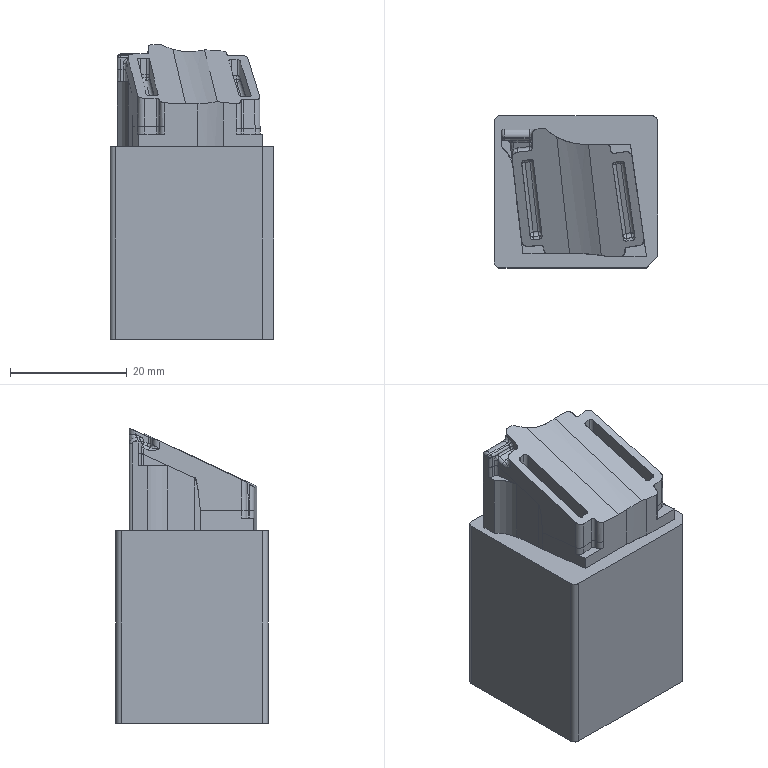NC program | NX | posted with a generic post | part box 28 x 26 x 50.455 mm
Lines 1 to 1095 of 4248:
N10 G17 G21 G94 G90
(CAVITY_MILL , TOOL : D6)
N12 T00 M6
N14 G54
N16 G17 G0 G90 X5.189 Y-18.995 S0 M3
N18 G43 Z10. H0
N20 Z-0.048
N22 G94 G1 Z-0.348 F250.
N24 Y-16.295
N26 G3 X2.189 Y-13.295 R3.
N28 G1 X-14.003
N30 G2 X-14.296 Y-13.002 R0.293
N32 G1 Y13.007
N34 G2 X-14.008 Y13.295 R0.288
N36 G1 X-10.132
N38 G2 X-6.501 Y14.818 R5.101
N40 G1 X-5.218
N42 G2 X-2.444 Y13.737 R4.1
N44 G3 X-2.084 Y13.432 R5.9
N46 G2 X-1.909 Y13.295 R4.185
N48 G1 X14.005
N50 G2 X14.295 Y13.005 R0.29
N52 G1 Y-13.008
N54 G2 X14.008 Y-13.295 R0.287
N56 G1 X2.189
N58 Y-10.295
N60 X-11.296
N62 Y8.229
N64 G3 X-7.035 Y5.647 R4.178
N66 G1 X-3.905 Y6.01
N68 X-3.886 Y6.012
N70 X-3.675 Y6.043
N72 X-3.539 Y6.08
N74 X-2.274 Y6.586
N76 X-2.149 Y6.654
N78 G3 X-0.393 Y10.295 R4.185
N80 G1 X-0.992 Y10.262
N82 G2 X-2.497 Y7.143 R3.585
N84 G1 X-3.762 Y6.637
N86 X-3.974 Y6.606
N88 X-7.104 Y6.243
N90 G2 X-10.881 Y10.738 R3.578
N92 G1 X-10.873 Y10.762
N94 X-10.85 Y10.862
N96 G2 X-6.501 Y14.218 R4.501
N98 G1 X-5.218
N100 G2 X-2.85 Y13.295 R3.5
N102 G3 X-2.447 Y12.954 R6.5
N104 G2 X-0.992 Y10.262 R3.585
N106 G1 X-0.393 Y10.295
N108 X11.295
N110 Y-10.295
N112 X2.189
N114 Y-7.295
N116 X-8.296
N118 Y2.681
N120 G3 X-6.689 Y2.667 R7.178
N122 G1 X-3.536 Y3.032
N124 X-3.472 Y3.041
N126 X-3.237 Y3.075
N128 G3 X-2.426 Y3.294 R3.6
N130 G1 X-1.16 Y3.8
N132 G3 X-0.412 Y4.208 R3.6
N134 X2.057 Y7.295 R7.185
N136 G1 X8.295
N138 Y-7.295
N140 X2.189
N142 Y-4.295
N144 X-5.296
N146 Y-0.192
N148 X-3.167 Y0.055
N150 X-3.057 Y0.07
N152 X-2.8 Y0.107
N154 G3 X-1.312 Y0.509 R6.6
N156 G1 X-0.046 Y1.015
N158 G3 X1.324 Y1.761 R6.6
N160 X3.82 Y4.295 R10.185
N162 G1 X5.295
N164 Y-4.295
N166 X2.189
N168 Y-1.295
N170 X2.082
N172 G3 X2.295 Y-1.176 R9.6
N174 G1 Y-1.295
N176 X2.189
N178 G3 X-0.811 Y-4.295 R3.
N180 G1 Z-0.048
N182 G0 Z0.3
N184 X3. Y-18.995
N186 Z-0.395
N188 G1 Z-0.695
N190 Y-16.295
N192 G3 X0. Y-13.295 R3.
N194 G1 X-14.003
N196 G2 X-14.296 Y-13.002 R0.293
N198 G1 Y13.007
N200 G2 X-14.008 Y13.295 R0.288
N202 G1 X-10.137
N204 G2 X-6.502 Y14.818 R5.1
N206 G1 X-5.218
N208 G2 X-2.444 Y13.737 R4.1
N210 G3 X-1.902 Y13.295 R5.9
N212 G1 X14.005
N214 G2 X14.295 Y13.005 R0.291
N216 G1 Y-13.008
N218 G2 X14.008 Y-13.295 R0.287
N220 G1 X0.
N222 Y-10.295
N224 X-11.296
N226 Y7.474
N228 G3 X-7.036 Y4.896 R4.166
N230 G1 X-2.8 Y5.387
N232 G3 X0.043 Y7.269 R3.77
N234 X0.495 Y10.295 R4.247
N236 G1 X-0.09 Y10.164
N238 G2 X-0.479 Y7.566 R3.647
N240 X-2.87 Y5.983 R3.17
N242 G1 X-7.105 Y5.492
N244 G2 X-11.002 Y9.102 R3.566
N246 G1 Y9.712
N248 G2 X-6.502 Y14.218 R4.5
N250 G1 X-5.218
N252 G2 X-2.85 Y13.295 R3.5
N254 G3 X-1.843 Y12.536 R6.5
N256 G2 X-0.09 Y10.164 R3.647
N258 G1 X0.495 Y10.295
N260 X11.295
N262 Y-10.295
N264 X0.
N266 Y-7.295
N268 X-8.296
N270 Y1.928
N272 G3 X-6.69 Y1.916 R7.166
N274 G1 X-2.455 Y2.407
N276 G3 X2.651 Y5.786 R6.77
N278 X3.295 Y7.295 R7.247
N280 G1 X8.295
N282 Y-7.295
N284 X0.
N286 Y-4.295
N288 X-5.296
N290 Y-0.942
N292 X-2.109 Y-0.573
N294 G3 X5.254 Y4.295 R9.77
N296 G1 X5.295
N298 Y-4.295
N300 X0.
N302 G3 X-3. Y-7.295 R3.
N304 G1 Y-18.995
N306 Z-0.395
N308 G0 Z-0.048
N310 X3.
N312 Z-0.743
N314 G1 Z-1.043
N316 Y-16.295
N318 G3 X0. Y-13.295 R3.
N320 G1 X-14.003
N322 G2 X-14.296 Y-13.002 R0.293
N324 G1 Y13.007
N326 G2 X-14.008 Y13.295 R0.288
N328 G1 X-10.152
N330 G2 X-6.527 Y14.818 R5.078
N332 G1 X-5.218
N334 G2 X-2.444 Y13.737 R4.1
N336 G3 X-1.902 Y13.295 R5.9
N338 G1 X14.005
N340 G2 X14.295 Y13.005 R0.291
N342 G1 Y-13.008
N344 G2 X14.008 Y-13.295 R0.287
N346 G1 X0.
N348 Y-10.295
N350 X-11.296
N352 Y6.715
N354 G3 X-7.049 Y4.144 R4.158
N356 G1 X-2.772 Y4.64
N358 X-1.197 Y4.728
N360 X-1.175 Y4.73
N362 G3 X2.695 Y3.609 R6.725
N364 G1 X2.767 Y3.615
N366 X5.869 Y4.063
N368 G3 X8.649 Y10.295 R4.048
N370 G1 X8.149 Y9.965
N372 G2 X5.784 Y4.657 R3.448
N374 G1 X2.681 Y4.209
N376 G2 X-1.038 Y5.365 R6.125
N378 G1 X-1.231 Y5.327
N380 X-2.823 Y5.238
N382 X-7.106 Y4.741
N384 G2 X-11.003 Y8.351 R3.558
N386 G1 X-11.004 Y9.735
N388 G2 X-6.527 Y14.218 R4.478
N390 G1 X-5.218
N392 G2 X-2.85 Y13.295 R3.5
N394 G3 X-1.029 Y12.114 R6.5
N396 G2 X0.187 Y11.424 R5.654
N398 G1 X1.3 Y11.576
N400 X1.574 Y11.581
N402 X4.049
N404 G2 X5.73 Y11.483 R10.39
N406 X8.149 Y9.965 R3.448
N408 G1 X8.649 Y10.295
N410 X11.295
N412 Y-10.295
N414 X0.
N416 Y-7.295
N418 X-8.296
N420 Y1.176
N422 G3 X-6.703 Y1.164 R7.158
N424 G1 X-2.515 Y1.65
N426 X-1.903 Y1.684
N428 G3 X2.761 Y0.61 R9.725
N430 X3.196 Y0.646 R3.6
N432 G1 X6.313 Y1.096
N434 G3 X8.295 Y1.701 R7.048
N436 G1 Y-7.295
N438 X0.
N440 Y-4.295
N442 X-5.296
N444 Y-1.693
N446 X-2.466 Y-1.365
N448 G3 X2.828 Y-2.39 R12.725
N450 X3.625 Y-2.324 R6.6
N452 G1 X5.295 Y-2.082
N454 Y-4.295
N456 X0.
N458 G3 X-3. Y-7.295 R3.
N460 G1 Y-18.995
N462 Z-0.743
N464 G0 Z-0.395
N466 X3.
N468 Z-1.091
N470 G1 Z-1.391
N472 Y-16.295
N474 G3 X0. Y-13.295 R3.
N476 G1 X-14.003
N478 G2 X-14.296 Y-13.002 R0.293
N480 G1 Y13.007
N482 G2 X-14.008 Y13.295 R0.288
N484 G1 X-10.241
N486 G2 X-6.557 Y14.818 R5.166
N488 G1 X-5.218
N490 G2 X-2.444 Y13.737 R4.1
N492 G3 X-1.902 Y13.295 R5.9
N494 G1 X14.005
N496 G2 X14.296 Y13.004 R0.291
N498 G1 X14.295 Y-13.008
N500 G2 X14.008 Y-13.295 R0.287
N502 G1 X0.
N504 Y-10.295
N506 X-11.296
N508 Y5.957
N510 G3 X-7.049 Y3.393 R4.154
N512 G1 X-2.681 Y3.9
N514 G2 X0.39 Y3.283 R5.63
N516 G3 X2.853 Y2.871 R4.182
N518 G1 X6.498 Y3.398
N520 G3 X9.902 Y8.337 R4.126
N522 X8.986 Y10.295 R4.882
N524 G1 X8.513 Y9.927
N526 G2 X9.315 Y8.211 R4.282
N528 X6.412 Y3.992 R3.526
N530 G1 X2.767 Y3.465
N532 G2 X0.668 Y3.816 R3.582
N534 G3 X-2.741 Y4.497 R6.23
N536 G1 X-7.118 Y3.989
N538 G2 X-11.004 Y7.6 R3.554
N540 G1 X-11.005 Y8.547
N542 G2 X-10.003 Y12.676 R4.399
N544 G1 X-9.932 Y12.751
N546 G2 X-6.558 Y14.218 R4.566
N548 G1 X-5.218
N550 G2 X-2.85 Y13.295 R3.5
N552 G3 X1.548 Y11.581 R6.5
N554 G1 X5.214
N556 G2 X8.513 Y9.927 R4.282
N558 G1 X8.986 Y10.295
N560 X11.296
N562 X11.295 Y-10.295
N564 X0.
N566 Y-7.295
N568 X-8.296
N570 Y0.424
N572 G3 X-6.73 Y0.41 R7.154
N574 G1 X-2.392 Y0.914
N576 G2 X-0.98 Y0.615 R2.63
N578 G3 X3.282 Y-0.098 R7.182
N580 G1 X6.942 Y0.431
N582 G3 X8.295 Y0.776 R7.126
N584 G1 Y-7.295
N586 X0.
N588 Y-4.295
N590 X-5.296
N592 Y-2.444
N594 X-2.274 Y-2.093
N596 G3 X3.711 Y-3.067 R10.182
N598 G1 X5.295 Y-2.838
N600 Y-4.295
N602 X0.
N604 G3 X-3. Y-7.295 R3.
N606 G1 Y-18.995
N608 Z-1.091
N610 G0 Z-0.743
N612 X3.
N614 Z-1.439
N616 G1 Z-1.739
N618 Y-16.295
N620 G3 X0. Y-13.295 R3.
N622 G1 X-14.003
N624 G2 X-14.296 Y-13.002 R0.293
N626 G1 Y4.317
N628 G2 X-14.788 Y5.842 R4.061
N630 X-14.893 Y13.48 R4.82
N632 G1 X-14.87 Y13.497
N634 G2 X-12.281 Y14.37 R4.652
N636 G1 X-12.265
N638 X-8.86
N640 G2 X-6.684 Y14.818 R5.5
N642 G1 X-5.218
N644 G2 X-2.444 Y13.737 R4.1
N646 G3 X-1.902 Y13.295 R5.9
N648 G1 X14.005
N650 G2 X14.296 Y13.004 R0.291
N652 G1 X14.295 Y-13.008
N654 G2 X14.008 Y-13.295 R0.287
N656 G1 X0.
N658 Y-10.295
N660 X-11.296
N662 Y2.277
N664 G3 X-10.302 Y2.265 R4.061
N666 G1 X-2.6 Y3.159
N668 G2 X0.39 Y2.576 R5.606
N670 G3 X2.94 Y2.128 R4.291
N672 G1 X6.683 Y2.668
N674 G3 X10.03 Y7.68 R3.999
N676 X8.991 Y10.295 R4.946
N678 G1 X8.52 Y9.924
N680 G2 X9.437 Y7.574 R4.346
N682 X6.602 Y3.263 R3.399
N684 G1 X2.854 Y2.722
N686 G2 X0.664 Y3.109 R3.691
N688 G3 X-2.66 Y3.756 R6.206
N690 G1 X-10.372 Y2.861
N692 G2 X-14.211 Y6.171 R3.461
N694 X-14.52 Y13.01 R4.22
N696 X-12.265 Y13.77 R4.052
N698 G1 X-8.733
N700 G2 X-6.684 Y14.218 R4.9
N702 G1 X-5.218
N704 G2 X-2.85 Y13.295 R3.5
N706 G3 X1.548 Y11.581 R6.5
N708 G1 X5.214
N710 G2 X8.52 Y9.924 R4.346
N712 G1 X8.991 Y10.295
N714 X11.296
N716 X11.295 Y-10.295
N718 X0.
N720 Y-7.295
N722 X-8.296
N724 Y-0.522
N726 X-2.313 Y0.172
N728 G2 X-0.975 Y-0.096 R2.606
N730 G3 X3.368 Y-0.842 R7.291
N732 G1 X7.093 Y-0.304
N734 G3 X8.295 Y-0.034 R6.999
N736 G1 Y-7.295
N738 X0.
N740 Y-4.295
N742 X-5.296
N744 Y-3.194
N746 X-2.205 Y-2.835
N748 G3 X3.797 Y-3.811 R10.291
N750 G1 X5.295 Y-3.594
N752 Y-4.295
N754 X0.
N756 G3 X-3. Y-7.295 R3.
N758 G1 Y-18.995
N760 Z-1.439
N762 G0 Z-1.091
N764 X0.236
N766 Z-1.786
N768 G1 Z-2.086
N770 Y-16.295
N772 G3 X-2.764 Y-13.295 R3.
N774 G1 X-14.003
N776 G2 X-14.296 Y-13.002 R0.293
N778 G1 Y3.277
N780 G2 X-15.036 Y5.616 R4.172
N782 X-16.56 Y7.708 R4.717
N784 G1 X-16.571 Y7.74
N786 G2 X-16.763 Y10.866 R6.746
N788 X-12.271 Y14.677 R4.606
N790 G1 X-12.265
N792 X-8.229
N794 X-8.104 Y14.703
N796 X-8.046 Y14.713
N798 X-7.115 Y14.814
N800 X-7.05 Y14.818
N802 X-5.218
N804 G2 X-2.444 Y13.737 R4.1
N806 G3 X-1.902 Y13.295 R5.9
N808 G1 X14.005
N810 G2 X14.296 Y13.004 R0.291
N812 G1 Y10.154
N814 X11.296
N816 G3 X11.061 Y10.295 R5.014
N818 G1 X11.296
N820 Y10.154
N822 X14.296
N824 X14.295 Y-13.008
N826 G2 X14.008 Y-13.295 R0.287
N828 G1 X-2.764
N830 Y-10.295
N832 X-11.296
N834 Y1.5
N836 G3 X-10.446 Y1.498 R4.172
N838 G1 X-2.52 Y2.418
N840 G2 X0.394 Y1.866 R5.581
N842 G3 X3.026 Y1.384 R4.407
N844 G1 X9.987 Y2.39
N846 G3 X11.296 Y2.832 R4.107
N848 G1 X11.01 Y3.36
N850 G2 X9.901 Y2.983 R3.507
N852 G1 X2.94 Y1.978
N854 G2 X0.668 Y2.4 R3.807
N856 G3 X-2.579 Y3.015 R6.181
N858 G1 X-10.515 Y2.094
N860 G2 X-14.426 Y5.915 R3.572
N862 X-15.997 Y7.915 R4.117
N864 X-16.172 Y10.762 R6.146
N866 X-12.265 Y14.077 R4.006
N868 G1 X-8.167
N870 X-7.981 Y14.116
N872 X-7.05 Y14.218
N874 X-5.218
N876 G2 X-2.85 Y13.295 R3.5
N878 G3 X1.548 Y11.581 R6.5
N880 G1 X5.214
N882 G2 X8.173 Y10.322 R4.35
N884 X12.374 Y8.211 R4.414
N886 X11.01 Y3.36 R3.507
N888 G1 X11.296 Y2.832
N890 X11.295 Y-10.295
N892 X-2.764
N894 Y-7.295
N896 X-8.296
N898 Y-1.273
N900 X-2.234 Y-0.569
N902 G2 X-0.959 Y-0.812 R2.581
N904 G3 X3.455 Y-1.585 R7.407
N906 G1 X8.295 Y-0.886
N908 Y-7.295
N910 X-2.764
N912 Y-4.295
N914 X-5.296
N916 Y-3.945
N918 X-2.137 Y-3.578
N920 G3 X-0.233 Y-4.295 R10.407
N922 G1 X-2.764
N924 G3 X-5.764 Y-7.295 R3.
N926 G1 Y-18.995
N928 Z-1.786
N930 G0 Z-1.439
N932 X-0.112
N934 Z-2.134
N936 G1 Z-2.434
N938 Y-16.295
N940 G3 X-3.112 Y-13.295 R3.
N942 G1 X-14.003
N944 G2 X-14.296 Y-13.002 R0.293
N946 G1 Y2.678
N948 G2 X-14.919 Y4.48 R4.168
N950 G1 X-14.997 Y5.13
N952 X-15.001 Y5.178
N954 X-15.015 Y5.542
N956 G2 X-16.498 Y7.415 R4.665
N958 G1 X-16.507 Y7.439
N960 X-16.635 Y7.769
N962 X-16.654 Y7.828
N964 X-16.708 Y8.028
N966 X-16.717 Y8.068
N968 X-16.778 Y8.262
N970 X-16.802 Y8.381
N972 X-16.862 Y8.99
N974 X-16.865 Y9.048
N976 Y10.194
N978 Y10.2
N980 G2 X-12.272 Y14.801 R4.646
N982 G1 X-12.265
N984 X-8.019
N986 X-7.335 Y14.817
N988 X-7.321 Y14.818
N990 X-5.218
N992 G2 X-2.444 Y13.737 R4.1
N994 G3 X-1.902 Y13.295 R5.9
N996 G1 X14.005
N998 G2 X14.296 Y13.004 R0.291
N1000 G1 Y10.158
N1002 X11.296
N1004 G3 X11.064 Y10.295 R5.099
N1006 G1 X11.296
N1008 Y10.158
N1010 X14.296
N1012 X14.295 Y-13.008
N1014 G2 X14.008 Y-13.295 R0.287
N1016 G1 X-3.112
N1018 Y-10.295
N1020 X-11.296
N1022 Y0.77
N1024 G3 X-10.36 Y0.758 R4.168
N1026 G1 X-8.832 Y0.935
N1028 X-8.691 Y0.969
N1030 G2 X-7.784 Y1.143 R2.763
N1032 G1 X-6.891 Y1.163
N1034 X-6.835 Y1.167
N1036 X-2.437 Y1.677
N1038 G2 X0.58 Y1.066 R5.541
N1040 G3 X3.092 Y0.638 R4.147
N1042 G1 X10.19 Y1.663
N1044 G3 X11.296 Y1.997 R4.143
N1046 G1 X11.043 Y2.542
N1048 G2 X10.104 Y2.257 R3.543
N1050 G1 X3.007 Y1.232
N1052 G2 X0.858 Y1.598 R3.547
N1054 G3 X-2.497 Y2.274 R6.141
N1056 G1 X-6.904 Y1.763
N1058 X-7.797 Y1.743
N1060 G3 X-8.901 Y1.531 R3.363
N1062 G1 X-10.429 Y1.354
N1064 G2 X-14.323 Y4.547 R3.568
N1066 G1 X-14.401 Y5.202
N1068 X-14.428 Y5.864
N1070 G2 X-15.948 Y7.655 R4.065
N1072 G1 X-16.075 Y7.985
N1074 X-16.129 Y8.186
N1076 X-16.13 Y8.198
N1078 X-16.205 Y8.44
N1080 X-16.265 Y9.048
N1082 Y10.194
N1084 G2 X-12.265 Y14.201 R4.046
N1086 G1 X-8.012
N1088 X-7.321 Y14.218
N1090 X-5.218
N1092 G2 X-2.85 Y13.295 R3.5
N1094 G3 X1.548 Y11.581 R6.5
N1096 G1 X5.214
N1098 G2 X8.172 Y10.325 R4.35
N1100 X13.031 Y6.478 R4.499
N1102 G1 X13.056 Y6.298
N1104 G2 X11.043 Y2.542 R3.543
N1106 G1 X11.296 Y1.997
N1108 X11.295 Y-10.295
N1110 X-3.112
N1112 Y-7.295
N1114 X-8.296
N1116 Y-2.018
N1118 G3 X-7.679 Y-1.855 R3.6
N1120 G1 X-6.825 Y-1.837
N1122 G3 X-6.489 Y-1.813 R3.6
N1124 G1 X-2.151 Y-1.31
N1126 G2 X-0.808 Y-1.593 R2.541
N1128 G3 X3.521 Y-2.331 R7.147
N1130 G1 X8.296 Y-1.642
N1132 X8.295 Y-7.295
N1134 X-3.112
N1136 Y-4.595
N1138 X-5.596
N1140 Y-4.428
N1142 X-2.009 Y-4.012
N1144 G3 X-0.627 Y-4.595 R9.847
N1146 G1 X-3.112
N1148 G3 X-6.112 Y-7.595 R3.
N1150 G1 Y-18.995
N1152 Z-2.134
N1154 G0 Z-1.786
N1156 X3.
N1158 Z-2.482
N1160 G1 Z-2.782
N1162 Y-16.295
N1164 G3 X0. Y-13.295 R3.
N1166 G1 X-14.003
N1168 G2 X-14.296 Y-13.002 R0.293
N1170 G1 Y2.1
N1172 G2 X-14.669 Y3.043 R4.064
N1174 G1 X-14.671 Y3.052
N1176 X-14.82 Y3.665
N1178 X-14.832 Y3.734
N1180 X-15. Y5.131
N1182 X-15.004 Y5.18
N1184 X-15.018 Y5.541
N1186 G2 X-16.501 Y7.422 R4.674
N1188 G1 X-16.51 Y7.445
N1190 X-16.634 Y7.767
N1192 X-16.654 Y7.829
N1194 X-16.71 Y8.04
N1196 X-16.788 Y8.317
N1198 X-16.808 Y8.423
N1200 X-16.854 Y8.915
N1202 X-16.865 Y9.028
N1204 Y10.218
N1206 G2 X-12.265 Y14.818 R4.6
N1208 G1 X-5.218
N1210 G2 X-2.444 Y13.737 R4.1
N1212 G3 X-1.902 Y13.295 R5.9
N1214 G1 X14.005
N1216 G2 X14.296 Y13.004 R0.291
N1218 G1 Y10.161
N1220 X11.296
N1222 G3 X11.07 Y10.295 R5.099
N1224 G1 X11.296
N1226 Y10.161
N1228 X14.296
N1230 X14.295 Y-13.008
N1232 G2 X14.008 Y-13.295 R0.287
N1234 G1 X0.
N1236 Y-10.295
N1238 X-11.296
N1240 Y0.03
N1242 G3 X-10.274 Y0.017 R4.064
N1244 G1 X-8.764 Y0.192
N1246 X-8.675 Y0.209
N1248 X-7.763 Y0.459
N1250 X-6.818 Y0.425
N1252 X-6.728 Y0.429
N1254 X-2.357 Y0.936
N1256 G2 X0.651 Y0.325 R5.503
N1258 G3 X3.173 Y-0.107 R4.154
N1260 G1 X6.849 Y0.424
N1262 X6.937 Y0.444
N1264 X7.839 Y0.717
N1266 X8.781 Y0.71
N1268 X8.871 Y0.716
N1270 X10.297 Y0.922
N1272 G3 X11.296 Y1.231 R4.238
N1274 G1 X11.049 Y1.778
N1276 G2 X10.211 Y1.516 R3.638
N1278 G1 X8.785 Y1.31
N1280 X7.752 Y1.318
N1282 X6.763 Y1.018
N1284 X3.087 Y0.487
N1286 G2 X0.929 Y0.857 R3.554
N1288 G3 X-2.416 Y1.533 R6.103
N1290 G1 X-6.797 Y1.025
N1292 X-7.833 Y1.061
N1294 X-8.833 Y0.788
N1296 X-10.343 Y0.613
N1298 G2 X-14.088 Y3.193 R3.464
N1300 G1 X-14.237 Y3.806
N1302 X-14.405 Y5.203
N1304 X-14.429 Y5.862
N1306 G2 X-15.95 Y7.661 R4.074
N1308 G1 X-16.074 Y7.983
N1310 X-16.131 Y8.198
N1312 X-16.21 Y8.48
N1314 X-16.262 Y9.028
N1316 X-16.265
N1318 Y10.218
N1320 G2 X-12.265 Y14.218 R4.
N1322 G1 X-5.218
N1324 G2 X-2.85 Y13.295 R3.5
N1326 G3 X1.548 Y11.581 R6.5
N1328 G1 X5.214
N1330 G2 X8.172 Y10.327 R4.349
N1332 X13.032 Y6.48 R4.499
N1334 G1 X13.156 Y5.607
N1336 G2 X11.049 Y1.778 R3.638
N1338 G1 X11.296 Y1.231
N1340 X11.295 Y-10.295
N1342 X0.
N1344 Y-7.295
N1346 X-8.296
N1348 Y-2.771
N1350 G3 X-7.885 Y-2.685 R3.6
N1352 G1 X-7.413 Y-2.556
N1354 X-6.925 Y-2.573
N1356 G3 X-6.382 Y-2.551 R3.6
N1358 G1 X-2.07 Y-2.051
N1360 G2 X-0.742 Y-2.332 R2.503
N1362 G3 X3.602 Y-3.076 R7.154
N1364 G1 X7.278 Y-2.545
N1366 G3 X7.806 Y-2.427 R3.6
N1368 G1 X8.273 Y-2.286
N1370 X8.296
N1372 X8.295 Y-7.295
N1374 X0.
N1376 G3 X-3. Y-10.295 R3.
N1378 G1 Y-18.995
N1380 Z-2.482
N1382 G0 Z-2.134
N1384 X3.
N1386 Z-2.83
N1388 G1 Z-3.13
N1390 Y-16.295
N1392 G3 X0. Y-13.295 R3.
N1394 G1 X-14.003
N1396 G2 X-14.296 Y-13.002 R0.293
N1398 G1 Y1.522
N1400 G2 X-14.747 Y2.996 R4.209
N1402 G1 X-15.004 Y5.133
N1404 X-15.007 Y5.167
N1406 X-15.031 Y5.551
N1408 G2 X-16.507 Y7.439 R4.639
N1410 G1 X-16.515 Y7.458
N1412 X-16.633 Y7.765
N1414 X-16.648 Y7.808
N1416 G2 X-16.854 Y8.913 R5.209
N1418 G1 X-16.865 Y9.028
N1420 Y10.218
N1422 G2 X-12.265 Y14.818 R4.6
N1424 G1 X-5.218
N1426 G2 X-2.444 Y13.737 R4.1
N1428 G3 X-1.902 Y13.295 R5.9
N1430 G1 X14.005
N1432 G2 X14.296 Y13.004 R0.291
N1434 G1 Y10.163
N1436 X11.296
N1438 G3 X11.074 Y10.295 R5.1
N1440 G1 X11.296
N1442 Y10.163
N1444 X14.296
N1446 X14.295 Y-13.008
N1448 G2 X14.008 Y-13.295 R0.288
N1450 G1 X0.
N1452 Y-10.295
N1454 X-11.296
N1456 Y-0.676
N1458 G3 X-10.188 Y-0.723 R4.209
N1460 G1 X-8.678 Y-0.548
N1462 X-8.589 Y-0.531
N1464 X-7.677 Y-0.282
N1466 X-6.732 Y-0.316
N1468 X-6.642 Y-0.312
N1470 X-2.282 Y0.194
N1472 G2 X0.913 Y-0.464 R6.274
N1474 G3 X3.276 Y-0.848 R3.99
N1476 G1 X6.956 Y-0.316
N1478 X7.044 Y-0.297
N1480 X7.946 Y-0.024
N1482 X8.888 Y-0.03
N1484 X8.978 Y-0.024
N1486 X10.404 Y0.182
N1488 G3 X11.296 Y0.431 R4.177
N1490 G1 X11.071 Y0.988
N1492 G2 X10.318 Y0.776 R3.577
N1494 G1 X8.892 Y0.57
N1496 X7.859 Y0.577
N1498 X6.87 Y0.278
N1500 X3.19 Y-0.254
N1502 G2 X1.183 Y0.073 R3.39
N1504 G3 X-2.335 Y0.792 R6.874
N1506 G1 X-6.711 Y0.284
N1508 X-7.747 Y0.321
N1510 X-8.747 Y0.048
N1512 X-10.257 Y-0.127
N1514 G2 X-14.151 Y3.065 R3.609
N1516 G1 X-14.408 Y5.204
N1518 X-14.45 Y5.876
N1520 G2 X-15.955 Y7.674 R4.039
N1522 G1 X-16.073 Y7.981
N1524 G2 X-16.26 Y9.028 R4.609
N1526 G1 X-16.265
N1528 Y10.218
N1530 G2 X-12.265 Y14.218 R4.
N1532 G1 X-5.218
N1534 G2 X-2.85 Y13.295 R3.5
N1536 G3 X1.548 Y11.581 R6.5
N1538 G1 X5.214
N1540 G2 X8.172 Y10.329 R4.348
N1542 X13.034 Y6.482 R4.5
N1544 G1 X13.263 Y4.866
N1546 G2 X11.071 Y0.988 R3.577
N1548 G1 X11.296 Y0.431
N1550 X11.295 Y-10.295
N1552 X0.
N1554 Y-7.295
N1556 X-8.296
N1558 Y-3.524
N1560 G3 X-7.799 Y-3.425 R3.6
N1562 G1 X-7.327 Y-3.296
N1564 X-6.839 Y-3.314
N1566 G3 X-6.296 Y-3.292 R3.6
N1568 G1 X-2.032 Y-2.797
N1570 G2 X-0.434 Y-3.144 R3.274
N1572 G3 X3.705 Y-3.817 R6.99
N1574 G1 X7.385 Y-3.285
N1576 G3 X7.913 Y-3.168 R3.6
N1578 G1 X8.296 Y-3.052
N1580 X8.295 Y-7.295
N1582 X0.
N1584 G3 X-3. Y-10.295 R3.
N1586 G1 Y-18.995
N1588 Z-2.83
N1590 G0 Z-2.482
N1592 X3.
N1594 Z-3.177
N1596 G1 Z-3.477
N1598 Y-16.295
N1600 G3 X0. Y-13.295 R3.
N1602 G1 X-14.003
N1604 G2 X-14.296 Y-13.002 R0.293
N1606 G1 Y0.977
N1608 G2 X-14.66 Y2.252 R4.245
N1610 G1 X-14.661 Y2.253
N1612 X-15.007 Y5.134
N1614 X-15.01 Y5.165
N1616 X-15.036 Y5.555
N1618 G2 X-16.514 Y7.456 R4.615
N1620 G1 X-16.521 Y7.472
N1622 X-16.633 Y7.763
N1624 X-16.647 Y7.805
N1626 G2 X-16.854 Y8.916 R5.181
N1628 G1 X-16.865 Y9.028
N1630 Y10.218
N1632 G2 X-12.265 Y14.818 R4.6
N1634 G1 X-5.218
N1636 G2 X-2.444 Y13.737 R4.1
N1638 G3 X-1.902 Y13.295 R5.9
N1640 G1 X14.005
N1642 G2 X14.296 Y13.004 R0.291
N1644 G1 Y10.166
N1646 X11.296
N1648 G3 X11.079 Y10.295 R5.101
N1650 G1 X11.296
N1652 Y10.166
N1654 X14.296
N1656 X14.295 Y-13.008
N1658 G2 X14.008 Y-13.295 R0.288
N1660 G1 X0.
N1662 Y-10.295
N1664 X-11.296
N1666 Y-1.393
N1668 G3 X-10.102 Y-1.464 R4.245
N1670 G1 X-8.592 Y-1.289
N1672 X-8.503 Y-1.272
N1674 X-7.629 Y-1.033
N1676 X-7.572 Y-1.037
N1678 X-6.637 Y-1.056
N1680 X-6.556 Y-1.053
N1682 X-2.206 Y-0.548
N1684 G2 X1.026 Y-1.225 R6.238
N1686 G3 X3.37 Y-1.59 R4.052
N1688 G1 X7.063 Y-1.057
N1690 X7.151 Y-1.037
N1692 X8.048 Y-0.766
N1694 X8.881 Y-0.784
N1696 X8.97 Y-0.779
N1698 X9.074 Y-0.766
N1700 X9.085 Y-0.765
N1702 X10.511 Y-0.559
N1704 G3 X11.296 Y-0.349 R4.187
N1706 G1 X11.085 Y0.213
N1708 G2 X10.425 Y0.035 R3.587
N1710 G1 X8.999 Y-0.171
N1712 X8.894 Y-0.184
N1714 X7.966 Y-0.164
N1716 X6.977 Y-0.463
N1718 X3.285 Y-0.996
N1720 G2 X1.3 Y-0.692 R3.452
N1722 G3 X-2.26 Y0.05 R6.838
N1724 G1 X-6.625 Y-0.457
N1726 X-7.559 Y-0.437
N1728 X-7.661 Y-0.42
N1730 X-8.661 Y-0.693
N1732 X-10.171 Y-0.868
N1734 G2 X-14.065 Y2.325 R3.645
N1736 G1 X-14.411 Y5.206
N1738 X-14.457 Y5.881
N1740 G2 X-15.961 Y7.688 R4.015
N1742 G1 X-16.073 Y7.979
N1744 G2 X-16.26 Y9.028 R4.581
N1746 G1 X-16.265
N1748 Y10.218
N1750 G2 X-12.265 Y14.218 R4.
N1752 G1 X-5.218
N1754 G2 X-2.85 Y13.295 R3.5
N1756 G3 X1.548 Y11.581 R6.5
N1758 G1 X5.214
N1760 G2 X8.171 Y10.331 R4.348
N1762 X13.035 Y6.484 R4.501
N1764 G1 X13.37 Y4.126
N1766 G2 X11.085 Y0.213 R3.587
N1768 G1 X11.296 Y-0.349
N1770 X11.295 Y-10.295
N1772 X0.
N1774 Y-7.295
N1776 X-8.296
N1778 Y-4.275
N1780 G3 X-7.713 Y-4.166 R3.6
N1782 G1 X-7.267 Y-4.044
N1784 X-6.7 Y-4.056
N1786 G3 X-6.21 Y-4.033 R3.6
N1788 G1 X-1.954 Y-3.539
N1790 G2 X-0.314 Y-3.91 R3.238
N1792 G3 X3.799 Y-4.559 R7.052
N1794 G1 X7.492 Y-4.026
N1796 G3 X8.02 Y-3.908 R3.6
N1798 G1 X8.296 Y-3.825
N1800 X8.295 Y-7.295
N1802 X0.
N1804 G3 X-3. Y-10.295 R3.
N1806 G1 Y-18.995
N1808 Z-3.177
N1810 G0 Z-2.83
N1812 X3.
N1814 Z-3.525
N1816 G1 Z-3.825
N1818 Y-16.295
N1820 G3 X0. Y-13.295 R3.
N1822 G1 X-14.003
N1824 G2 X-14.296 Y-13.002 R0.294
N1826 G1 Y0.388
N1828 G2 X-14.575 Y1.518 R4.168
N1830 G1 X-15.063 Y5.575
N1832 G2 X-16.675 Y7.907 R4.586
N1834 G1 X-16.679 Y7.922
N1836 X-16.715 Y8.055
N1838 X-16.727 Y8.108
N1840 X-16.839 Y8.745
N1842 X-16.846 Y8.805
N1844 X-16.854 Y8.916
N1846 X-16.865 Y9.028
N1848 Y10.218
N1850 G2 X-12.265 Y14.818 R4.6
N1852 G1 X-5.218
N1854 G2 X-2.444 Y13.737 R4.1
N1856 G3 X-1.902 Y13.295 R5.9
N1858 G1 X14.005
N1860 G2 X14.296 Y13.004 R0.291
N1862 G1 Y10.169
N1864 X11.296
N1866 G3 X11.084 Y10.295 R5.101
N1868 G1 X11.296
N1870 Y10.169
N1872 X14.296
N1874 X14.295 Y-13.008
N1876 G2 X14.008 Y-13.295 R0.288
N1878 G1 X0.
N1880 Y-10.295
N1882 X-11.296
N1884 Y-2.134
N1886 G3 X-10.016 Y-2.205 R4.168
N1888 G1 X-8.506 Y-2.029
N1890 X-8.43 Y-2.016
N1892 X-7.569 Y-1.801
N1894 X-7.465 Y-1.765
N1896 X-6.56 Y-1.797
N1898 X-6.47 Y-1.793
N1900 X-2.153 Y-1.292
N1902 G2 X1.031 Y-1.932 R6.203
N1904 G3 X3.457 Y-2.334 R4.094
N1906 G1 X7.17 Y-1.797
N1908 X7.258 Y-1.778
N1910 X8.16 Y-1.505
N1912 X9.101 Y-1.511
N1914 X9.191 Y-1.505
N1916 X10.618 Y-1.299
N1918 G3 X11.296 Y-1.131 R4.169
N1920 G1 X11.103 Y-0.563
N1922 G2 X10.532 Y-0.706 R3.569
N1924 G1 X9.106 Y-0.912
N1926 X8.073 Y-0.904
N1928 X7.084 Y-1.203
N1930 X3.371 Y-1.74
N1932 G2 X1.3 Y-1.396 R3.494
N1934 G3 X-2.208 Y-0.695 R6.803
N1936 G1 X-6.539 Y-1.197
N1938 X-7.575 Y-1.16
N1940 X-7.714 Y-1.218
N1942 X-8.575 Y-1.433
N1944 X-10.085 Y-1.609
N1946 G2 X-13.979 Y1.584 R3.568
N1948 G1 X-14.499 Y5.909
N1950 G2 X-16.1 Y8.079 R3.986
N1952 G1 X-16.136 Y8.211
N1954 X-16.248 Y8.849
N1956 X-16.261 Y9.028
N1958 X-16.265
N1960 Y10.218
N1962 G2 X-12.265 Y14.218 R4.
N1964 G1 X-5.218
N1966 G2 X-2.85 Y13.295 R3.5
N1968 G3 X1.548 Y11.581 R6.5
N1970 G1 X5.214
N1972 G2 X8.171 Y10.333 R4.348
N1974 X13.037 Y6.486 R4.501
N1976 G1 X13.477 Y3.385
N1978 G2 X11.103 Y-0.563 R3.569
N1980 G1 X11.296 Y-1.131
N1982 X11.295 Y-10.295
N1984 X0.
N1986 Y-7.295
N1988 X-8.296
N1990 Y-5.025
N1992 X-8.16 Y-5.009
N1994 G3 X-7.703 Y-4.926 R3.6
N1996 G1 X-7.114 Y-4.779
N1998 X-6.667 Y-4.795
N2000 G3 X-6.124 Y-4.773 R3.6
N2002 G1 X-1.892 Y-4.282
N2004 G2 X-0.315 Y-4.613 R3.203
N2006 G3 X3.886 Y-5.303 R7.094
N2008 G1 X7.599 Y-4.766
N2010 G3 X8.127 Y-4.649 R3.6
N2012 G1 X8.296 Y-4.598
N2014 Y-7.295
N2016 X0.
N2018 G3 X-3. Y-10.295 R3.
N2020 G1 Y-18.995
N2022 Z-3.525
N2024 G0 Z-3.177
N2026 X3.
N2028 Z-3.873
N2030 G1 Z-4.173
N2032 Y-16.295
N2034 G3 X0. Y-13.295 R3.
N2036 G1 X-14.003
N2038 G2 X-14.296 Y-13.002 R0.294
N2040 G1 Y-0.041
N2042 X-14.341 Y0.125
N2044 Y0.127
N2046 X-14.47 Y0.657
N2048 X-14.482 Y0.723
N2050 X-14.488 Y0.768
N2052 X-14.489 Y0.772
N2054 X-15.066 Y5.577
N2056 G2 X-16.441 Y7.291 R4.555
N2058 G1 X-16.46 Y7.336
N2060 X-16.685 Y7.951
N2062 X-16.702 Y8.004
N2064 X-16.726 Y8.098
N2066 X-16.737 Y8.15
N2068 X-16.839 Y8.748
N2070 X-16.846 Y8.805
N2072 X-16.854 Y8.916
N2074 X-16.865 Y9.028
N2076 Y10.218
N2078 G2 X-12.265 Y14.818 R4.6
N2080 G1 X-5.218
N2082 G2 X-2.444 Y13.737 R4.1
N2084 G3 X-1.902 Y13.295 R5.9
N2086 G1 X14.005
N2088 G2 X14.296 Y13.004 R0.291
N2090 G1 Y10.173
N2092 X11.296
N2094 G3 X11.09 Y10.295 R5.1
N2096 G1 X11.296
N2098 Y10.173
N2100 X14.296
N2102 X14.295 Y-13.008
N2104 G2 X14.008 Y-13.295 R0.288
N2106 G1 X0.
N2108 Y-10.295
N2110 X-11.296
N2112 Y-2.868
N2114 G3 X-9.93 Y-2.945 R4.071
N2116 G1 X-8.42 Y-2.77
N2118 X-8.338 Y-2.754
N2120 X-7.407 Y-2.511
N2122 X-7.385 Y-2.505
N2124 X-6.474 Y-2.537
N2126 X-6.384 Y-2.534
N2128 X-2.114 Y-2.038
N2130 G2 X1.028 Y-2.638 R6.033
N2132 G3 X3.543 Y-3.077 R4.184
N2134 G1 X7.277 Y-2.538
N2136 X7.353 Y-2.522
N2138 X8.209 Y-2.282
N2140 X8.283 Y-2.256
N2142 X9.215 Y-2.252
N2144 X9.298 Y-2.246
N2146 X10.725 Y-2.04
N2148 G3 X11.296 Y-1.905 R4.176
N2150 G1 X11.117 Y-1.332
N2152 G2 X10.639 Y-1.446 R3.576
N2154 G1 X9.213 Y-1.652
N2156 X8.261 Y-1.656
N2158 X8.18 Y-1.645
N2160 X8.048 Y-1.704
N2162 X7.191 Y-1.944
N2164 X3.458 Y-2.483
N2166 G2 X1.3 Y-2.103 R3.584
N2168 G3 X-2.173 Y-1.441 R6.633
N2170 G1 X-6.453 Y-1.938
N2172 X-7.489 Y-1.901
N2174 X-7.559 Y-1.931
N2176 X-8.489 Y-2.174
N2178 X-9.999 Y-2.349
N2180 G2 X-13.758 Y0.269 R3.471
N2182 G1 X-13.887 Y0.799
N2184 X-13.893 Y0.844
N2186 X-14.502 Y5.911
N2188 G2 X-15.896 Y7.542 R3.955